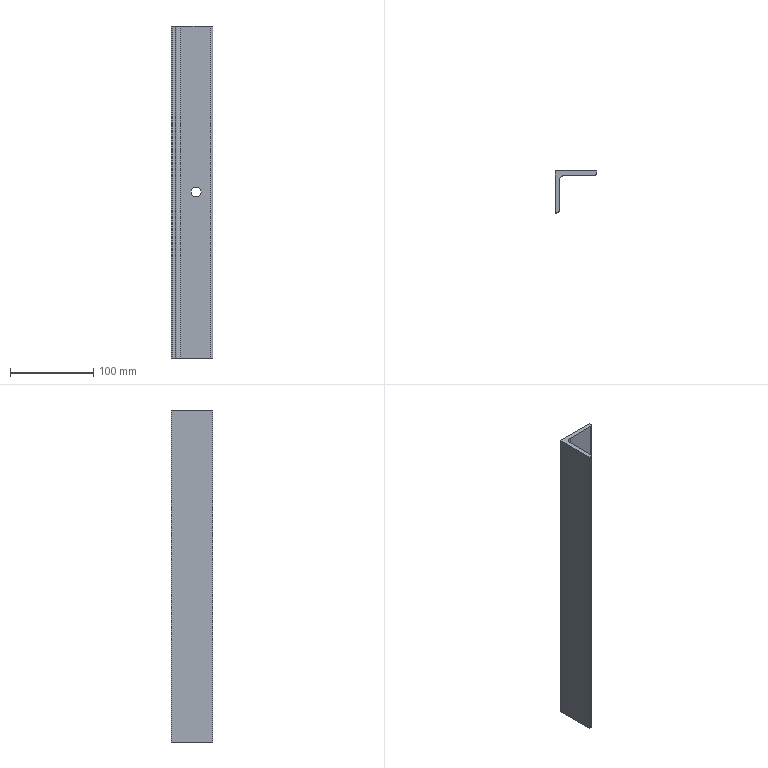Part | STEP file | Input 113 | 1 solid | 13 faces | box 50 x 50 x 400 mm | volume 191516 mm3 | plane 8 | cylinder 5 | commonest cylinder face diameters 6 x2 12 x2 13 x1
STEP:
#1=CARTESIAN_POINT('',(0.,0.,0.));
#2=DIRECTION('',(0.,0.,1.));
#3=DIRECTION('',(1.,0.,0.));
#4=AXIS2_PLACEMENT_3D('',#1,#2,#3);
#5=CARTESIAN_POINT('',(2984.,319.5,0.));
#6=VERTEX_POINT('',#5);
#7=CARTESIAN_POINT('',(2984.,324.5,0.));
#8=VERTEX_POINT('',#7);
#9=CARTESIAN_POINT('',(2984.,239.499,0.));
#10=DIRECTION('',(0.,1.,0.));
#11=VECTOR('',#10,1.);
#12=LINE('',#9,#11);
#13=CARTESIAN_POINT('',(2990.,239.499,0.));
#14=DIRECTION('',(0.,1.,0.));
#15=DIRECTION('',(-1.,0.,0.));
#16=AXIS2_PLACEMENT_3D('',#13,#14,#15);
#17=CYLINDRICAL_SURFACE('',#16,6.);
#18=CARTESIAN_POINT('',(6.283,0.));
#19=DIRECTION('',(0.,1.));
#20=VECTOR('',#19,1.);
#21=LINE('',#18,#20);
#22=(GEOMETRIC_REPRESENTATION_CONTEXT(2)PARAMETRIC_REPRESENTATION_CONTEXT()REPRESENTATION_CONTEXT('',''));
#23=DEFINITIONAL_REPRESENTATION('',(#21),#22);
#24=PCURVE('',#17,#23);
#25=CARTESIAN_POINT('',(2990.,239.499,0.));
#26=DIRECTION('',(0.,1.,0.));
#27=DIRECTION('',(-1.,0.,0.));
#28=AXIS2_PLACEMENT_3D('',#25,#26,#27);
#29=CYLINDRICAL_SURFACE('',#28,6.);
#30=CARTESIAN_POINT('',(0.,0.));
#31=DIRECTION('',(0.,1.));
#32=VECTOR('',#31,1.);
#33=LINE('',#30,#32);
#34=(GEOMETRIC_REPRESENTATION_CONTEXT(2)PARAMETRIC_REPRESENTATION_CONTEXT()REPRESENTATION_CONTEXT('',''));
#35=DEFINITIONAL_REPRESENTATION('',(#33),#34);
#36=PCURVE('',#29,#35);
#37=SURFACE_CURVE('',#12,(#24,#36),.PCURVE_S1.);
#38=EDGE_CURVE('',#6,#8,#37,.T.);
#39=ORIENTED_EDGE('',*,*,#38,.T.);
#40=CARTESIAN_POINT('',(2996.,324.5,0.));
#41=VERTEX_POINT('',#40);
#42=CARTESIAN_POINT('',(2990.,324.5,0.));
#43=DIRECTION('',(0.,1.,0.));
#44=DIRECTION('',(-1.,0.,0.));
#45=AXIS2_PLACEMENT_3D('',#42,#43,#44);
#46=CIRCLE('',#45,6.);
#47=CARTESIAN_POINT('',(0.,85.001));
#48=DIRECTION('',(1.,0.));
#49=VECTOR('',#48,1.);
#50=LINE('',#47,#49);
#51=(GEOMETRIC_REPRESENTATION_CONTEXT(2)PARAMETRIC_REPRESENTATION_CONTEXT()REPRESENTATION_CONTEXT('',''));
#52=DEFINITIONAL_REPRESENTATION('',(#50),#51);
#53=PCURVE('',#17,#52);
#54=CARTESIAN_POINT('',(3010.,324.5,200.));
#55=DIRECTION('',(0.,1.,0.));
#56=DIRECTION('',(-1.,0.,0.));
#57=AXIS2_PLACEMENT_3D('',#54,#55,#56);
#58=PLANE('',#57);
#59=CARTESIAN_POINT('',(20.,-200.));
#60=DIRECTION('',(1.,0.));
#61=AXIS2_PLACEMENT_2D('',#59,#60);
#62=CIRCLE('',#61,6.);
#63=(GEOMETRIC_REPRESENTATION_CONTEXT(2)PARAMETRIC_REPRESENTATION_CONTEXT()REPRESENTATION_CONTEXT('',''));
#64=DEFINITIONAL_REPRESENTATION('',(#62),#63);
#65=PCURVE('',#58,#64);
#66=SURFACE_CURVE('',#46,(#53,#65),.PCURVE_S1.);
#67=EDGE_CURVE('',#41,#8,#66,.T.);
#68=ORIENTED_EDGE('',*,*,#67,.F.);
#69=CARTESIAN_POINT('',(2996.,319.5,0.));
#70=VERTEX_POINT('',#69);
#71=CARTESIAN_POINT('',(2996.,239.499,0.));
#72=DIRECTION('',(0.,1.,0.));
#73=VECTOR('',#72,1.);
#74=LINE('',#71,#73);
#75=CARTESIAN_POINT('',(3.142,0.));
#76=DIRECTION('',(0.,1.));
#77=VECTOR('',#76,1.);
#78=LINE('',#75,#77);
#79=(GEOMETRIC_REPRESENTATION_CONTEXT(2)PARAMETRIC_REPRESENTATION_CONTEXT()REPRESENTATION_CONTEXT('',''));
#80=DEFINITIONAL_REPRESENTATION('',(#78),#79);
#81=PCURVE('',#17,#80);
#82=CARTESIAN_POINT('',(3.142,0.));
#83=DIRECTION('',(0.,1.));
#84=VECTOR('',#83,1.);
#85=LINE('',#82,#84);
#86=(GEOMETRIC_REPRESENTATION_CONTEXT(2)PARAMETRIC_REPRESENTATION_CONTEXT()REPRESENTATION_CONTEXT('',''));
#87=DEFINITIONAL_REPRESENTATION('',(#85),#86);
#88=PCURVE('',#29,#87);
#89=SURFACE_CURVE('',#74,(#81,#88),.PCURVE_S1.);
#90=EDGE_CURVE('',#70,#41,#89,.T.);
#91=ORIENTED_EDGE('',*,*,#90,.F.);
#92=CARTESIAN_POINT('',(2990.,319.5,0.));
#93=DIRECTION('',(0.,1.,0.));
#94=DIRECTION('',(1.,0.,0.));
#95=AXIS2_PLACEMENT_3D('',#92,#93,#94);
#96=CIRCLE('',#95,6.);
#97=CARTESIAN_POINT('',(3.142,80.001));
#98=DIRECTION('',(1.,0.));
#99=VECTOR('',#98,1.);
#100=LINE('',#97,#99);
#101=(GEOMETRIC_REPRESENTATION_CONTEXT(2)PARAMETRIC_REPRESENTATION_CONTEXT()REPRESENTATION_CONTEXT('',''));
#102=DEFINITIONAL_REPRESENTATION('',(#100),#101);
#103=PCURVE('',#17,#102);
#104=CARTESIAN_POINT('',(2971.5,319.5,200.));
#105=DIRECTION('',(0.,-1.,0.));
#106=DIRECTION('',(1.,0.,0.));
#107=AXIS2_PLACEMENT_3D('',#104,#105,#106);
#108=PLANE('',#107);
#109=CARTESIAN_POINT('',(24.5,-200.));
#110=CARTESIAN_POINT('',(24.5,-210.392));
#111=CARTESIAN_POINT('',(15.5,-205.196));
#112=CARTESIAN_POINT('',(6.5,-200.));
#113=CARTESIAN_POINT('',(15.5,-194.804));
#114=CARTESIAN_POINT('',(24.5,-189.608));
#115=CARTESIAN_POINT('',(24.5,-200.));
#116=(BOUNDED_CURVE()B_SPLINE_CURVE(2,(#109,#110,#111,#112,#113,#114,#115),.UNSPECIFIED.,.T.,.F.)B_SPLINE_CURVE_WITH_KNOTS((1,2,2,2,2,1),(-2.094,0.,2.094,4.189,6.283,8.378),.UNSPECIFIED.)CURVE()GEOMETRIC_REPRESENTATION_ITEM()RATIONAL_B_SPLINE_CURVE((1.,0.5,1.,0.5,1.,0.5,1.))REPRESENTATION_ITEM(''));
#117=(GEOMETRIC_REPRESENTATION_CONTEXT(2)PARAMETRIC_REPRESENTATION_CONTEXT()REPRESENTATION_CONTEXT('',''));
#118=DEFINITIONAL_REPRESENTATION('',(#116),#117);
#119=PCURVE('',#108,#118);
#120=SURFACE_CURVE('',#96,(#103,#119),.PCURVE_S1.);
#121=EDGE_CURVE('',#70,#6,#120,.T.);
#122=ORIENTED_EDGE('',*,*,#121,.T.);
#123=EDGE_LOOP('',(#39,#68,#91,#122));
#124=FACE_BOUND('',#123,.F.);
#125=ADVANCED_FACE('',(#124),#17,.F.);
#126=CARTESIAN_POINT('',(2990.,324.5,0.));
#127=DIRECTION('',(0.,1.,0.));
#128=DIRECTION('',(-1.,0.,0.));
#129=AXIS2_PLACEMENT_3D('',#126,#127,#128);
#130=CIRCLE('',#129,6.);
#131=CARTESIAN_POINT('',(20.,-200.));
#132=DIRECTION('',(1.,0.));
#133=AXIS2_PLACEMENT_2D('',#131,#132);
#134=CIRCLE('',#133,6.);
#135=(GEOMETRIC_REPRESENTATION_CONTEXT(2)PARAMETRIC_REPRESENTATION_CONTEXT()REPRESENTATION_CONTEXT('',''));
#136=DEFINITIONAL_REPRESENTATION('',(#134),#135);
#137=PCURVE('',#58,#136);
#138=CARTESIAN_POINT('',(0.,85.001));
#139=DIRECTION('',(1.,0.));
#140=VECTOR('',#139,1.);
#141=LINE('',#138,#140);
#142=(GEOMETRIC_REPRESENTATION_CONTEXT(2)PARAMETRIC_REPRESENTATION_CONTEXT()REPRESENTATION_CONTEXT('',''));
#143=DEFINITIONAL_REPRESENTATION('',(#141),#142);
#144=PCURVE('',#29,#143);
#145=SURFACE_CURVE('',#130,(#137,#144),.PCURVE_S1.);
#146=EDGE_CURVE('',#8,#41,#145,.T.);
#147=ORIENTED_EDGE('',*,*,#146,.F.);
#148=ORIENTED_EDGE('',*,*,#67,.F.);
#149=EDGE_LOOP('',(#147,#148));
#150=FACE_BOUND('',#149,.T.);
#151=CARTESIAN_POINT('',(2960.,324.5,-200.));
#152=VERTEX_POINT('',#151);
#153=CARTESIAN_POINT('',(3010.,324.5,-200.));
#154=VERTEX_POINT('',#153);
#155=CARTESIAN_POINT('',(3010.,324.5,-200.));
#156=DIRECTION('',(1.,0.,0.));
#157=VECTOR('',#156,1.);
#158=LINE('',#155,#157);
#159=CARTESIAN_POINT('',(0.,-400.));
#160=DIRECTION('',(-1.,0.));
#161=VECTOR('',#160,1.);
#162=LINE('',#159,#161);
#163=(GEOMETRIC_REPRESENTATION_CONTEXT(2)PARAMETRIC_REPRESENTATION_CONTEXT()REPRESENTATION_CONTEXT('',''));
#164=DEFINITIONAL_REPRESENTATION('',(#162),#163);
#165=PCURVE('',#58,#164);
#166=CARTESIAN_POINT('',(2962.,277.5,-200.));
#167=DIRECTION('',(0.,0.,1.));
#168=DIRECTION('',(1.,0.,0.));
#169=AXIS2_PLACEMENT_3D('',#166,#167,#168);
#170=PLANE('',#169);
#171=CARTESIAN_POINT('',(48.,47.));
#172=DIRECTION('',(1.,0.));
#173=VECTOR('',#172,1.);
#174=LINE('',#171,#173);
#175=(GEOMETRIC_REPRESENTATION_CONTEXT(2)PARAMETRIC_REPRESENTATION_CONTEXT()REPRESENTATION_CONTEXT('',''));
#176=DEFINITIONAL_REPRESENTATION('',(#174),#175);
#177=PCURVE('',#170,#176);
#178=SURFACE_CURVE('',#158,(#165,#177),.PCURVE_S1.);
#179=EDGE_CURVE('',#152,#154,#178,.T.);
#180=ORIENTED_EDGE('',*,*,#179,.F.);
#181=CARTESIAN_POINT('',(2960.,324.5,200.));
#182=VERTEX_POINT('',#181);
#183=CARTESIAN_POINT('',(2960.,324.5,200.));
#184=DIRECTION('',(0.,0.,-1.));
#185=VECTOR('',#184,1.);
#186=LINE('',#183,#185);
#187=CARTESIAN_POINT('',(50.,0.));
#188=DIRECTION('',(0.,-1.));
#189=VECTOR('',#188,1.);
#190=LINE('',#187,#189);
#191=(GEOMETRIC_REPRESENTATION_CONTEXT(2)PARAMETRIC_REPRESENTATION_CONTEXT()REPRESENTATION_CONTEXT('',''));
#192=DEFINITIONAL_REPRESENTATION('',(#190),#191);
#193=PCURVE('',#58,#192);
#194=CARTESIAN_POINT('',(2960.,324.5,200.));
#195=DIRECTION('',(-1.,0.,0.));
#196=DIRECTION('',(0.,0.,1.));
#197=AXIS2_PLACEMENT_3D('',#194,#195,#196);
#198=PLANE('',#197);
#199=CARTESIAN_POINT('',(0.,0.));
#200=DIRECTION('',(-1.,0.));
#201=VECTOR('',#200,1.);
#202=LINE('',#199,#201);
#203=(GEOMETRIC_REPRESENTATION_CONTEXT(2)PARAMETRIC_REPRESENTATION_CONTEXT()REPRESENTATION_CONTEXT('',''));
#204=DEFINITIONAL_REPRESENTATION('',(#202),#203);
#205=PCURVE('',#198,#204);
#206=SURFACE_CURVE('',#186,(#193,#205),.PCURVE_S1.);
#207=EDGE_CURVE('',#182,#152,#206,.T.);
#208=ORIENTED_EDGE('',*,*,#207,.F.);
#209=CARTESIAN_POINT('',(3010.,324.5,200.));
#210=VERTEX_POINT('',#209);
#211=CARTESIAN_POINT('',(3010.,324.5,200.));
#212=DIRECTION('',(1.,0.,0.));
#213=VECTOR('',#212,1.);
#214=LINE('',#211,#213);
#215=CARTESIAN_POINT('',(0.,0.));
#216=DIRECTION('',(-1.,0.));
#217=VECTOR('',#216,1.);
#218=LINE('',#215,#217);
#219=(GEOMETRIC_REPRESENTATION_CONTEXT(2)PARAMETRIC_REPRESENTATION_CONTEXT()REPRESENTATION_CONTEXT('',''));
#220=DEFINITIONAL_REPRESENTATION('',(#218),#219);
#221=PCURVE('',#58,#220);
#222=CARTESIAN_POINT('',(2962.,277.5,200.));
#223=DIRECTION('',(0.,0.,1.));
#224=DIRECTION('',(1.,0.,0.));
#225=AXIS2_PLACEMENT_3D('',#222,#223,#224);
#226=PLANE('',#225);
#227=CARTESIAN_POINT('',(48.,47.));
#228=DIRECTION('',(1.,0.));
#229=VECTOR('',#228,1.);
#230=LINE('',#227,#229);
#231=(GEOMETRIC_REPRESENTATION_CONTEXT(2)PARAMETRIC_REPRESENTATION_CONTEXT()REPRESENTATION_CONTEXT('',''));
#232=DEFINITIONAL_REPRESENTATION('',(#230),#231);
#233=PCURVE('',#226,#232);
#234=SURFACE_CURVE('',#214,(#221,#233),.PCURVE_S1.);
#235=EDGE_CURVE('',#182,#210,#234,.T.);
#236=ORIENTED_EDGE('',*,*,#235,.T.);
#237=CARTESIAN_POINT('',(3010.,324.5,200.));
#238=DIRECTION('',(0.,0.,-1.));
#239=VECTOR('',#238,1.);
#240=LINE('',#237,#239);
#241=CARTESIAN_POINT('',(0.,0.));
#242=DIRECTION('',(0.,-1.));
#243=VECTOR('',#242,1.);
#244=LINE('',#241,#243);
#245=(GEOMETRIC_REPRESENTATION_CONTEXT(2)PARAMETRIC_REPRESENTATION_CONTEXT()REPRESENTATION_CONTEXT('',''));
#246=DEFINITIONAL_REPRESENTATION('',(#244),#245);
#247=PCURVE('',#58,#246);
#248=CARTESIAN_POINT('',(3010.,324.5,200.));
#249=DIRECTION('',(1.,0.,0.));
#250=DIRECTION('',(0.,0.,-1.));
#251=AXIS2_PLACEMENT_3D('',#248,#249,#250);
#252=PLANE('',#251);
#253=CARTESIAN_POINT('',(0.,0.));
#254=DIRECTION('',(1.,0.));
#255=VECTOR('',#254,1.);
#256=LINE('',#253,#255);
#257=(GEOMETRIC_REPRESENTATION_CONTEXT(2)PARAMETRIC_REPRESENTATION_CONTEXT()REPRESENTATION_CONTEXT('',''));
#258=DEFINITIONAL_REPRESENTATION('',(#256),#257);
#259=PCURVE('',#252,#258);
#260=SURFACE_CURVE('',#240,(#247,#259),.PCURVE_S1.);
#261=EDGE_CURVE('',#210,#154,#260,.T.);
#262=ORIENTED_EDGE('',*,*,#261,.T.);
#263=EDGE_LOOP('',(#180,#208,#236,#262));
#264=FACE_BOUND('',#263,.T.);
#265=ADVANCED_FACE('',(#150,#264),#58,.T.);
#266=CARTESIAN_POINT('',(2960.,274.5,-200.));
#267=VERTEX_POINT('',#266);
#268=CARTESIAN_POINT('',(2960.,324.5,-200.));
#269=DIRECTION('',(0.,1.,0.));
#270=VECTOR('',#269,1.);
#271=LINE('',#268,#270);
#272=CARTESIAN_POINT('',(-400.,0.));
#273=DIRECTION('',(0.,1.));
#274=VECTOR('',#273,1.);
#275=LINE('',#272,#274);
#276=(GEOMETRIC_REPRESENTATION_CONTEXT(2)PARAMETRIC_REPRESENTATION_CONTEXT()REPRESENTATION_CONTEXT('',''));
#277=DEFINITIONAL_REPRESENTATION('',(#275),#276);
#278=PCURVE('',#198,#277);
#279=CARTESIAN_POINT('',(-2.,47.));
#280=DIRECTION('',(0.,1.));
#281=VECTOR('',#280,1.);
#282=LINE('',#279,#281);
#283=(GEOMETRIC_REPRESENTATION_CONTEXT(2)PARAMETRIC_REPRESENTATION_CONTEXT()REPRESENTATION_CONTEXT('',''));
#284=DEFINITIONAL_REPRESENTATION('',(#282),#283);
#285=PCURVE('',#170,#284);
#286=SURFACE_CURVE('',#271,(#278,#285),.PCURVE_S1.);
#287=EDGE_CURVE('',#267,#152,#286,.T.);
#288=ORIENTED_EDGE('',*,*,#287,.F.);
#289=CARTESIAN_POINT('',(2960.,274.5,200.));
#290=VERTEX_POINT('',#289);
#291=CARTESIAN_POINT('',(2960.,274.5,200.));
#292=DIRECTION('',(0.,0.,-1.));
#293=VECTOR('',#292,1.);
#294=LINE('',#291,#293);
#295=CARTESIAN_POINT('',(0.,-50.));
#296=DIRECTION('',(-1.,0.));
#297=VECTOR('',#296,1.);
#298=LINE('',#295,#297);
#299=(GEOMETRIC_REPRESENTATION_CONTEXT(2)PARAMETRIC_REPRESENTATION_CONTEXT()REPRESENTATION_CONTEXT('',''));
#300=DEFINITIONAL_REPRESENTATION('',(#298),#299);
#301=PCURVE('',#198,#300);
#302=CARTESIAN_POINT('',(2960.,274.5,200.));
#303=DIRECTION('',(0.,-1.,0.));
#304=DIRECTION('',(1.,0.,0.));
#305=AXIS2_PLACEMENT_3D('',#302,#303,#304);
#306=PLANE('',#305);
#307=CARTESIAN_POINT('',(0.,0.));
#308=DIRECTION('',(0.,-1.));
#309=VECTOR('',#308,1.);
#310=LINE('',#307,#309);
#311=(GEOMETRIC_REPRESENTATION_CONTEXT(2)PARAMETRIC_REPRESENTATION_CONTEXT()REPRESENTATION_CONTEXT('',''));
#312=DEFINITIONAL_REPRESENTATION('',(#310),#311);
#313=PCURVE('',#306,#312);
#314=SURFACE_CURVE('',#294,(#301,#313),.PCURVE_S1.);
#315=EDGE_CURVE('',#290,#267,#314,.T.);
#316=ORIENTED_EDGE('',*,*,#315,.F.);
#317=CARTESIAN_POINT('',(2960.,324.5,200.));
#318=DIRECTION('',(0.,1.,0.));
#319=VECTOR('',#318,1.);
#320=LINE('',#317,#319);
#321=CARTESIAN_POINT('',(0.,0.));
#322=DIRECTION('',(0.,1.));
#323=VECTOR('',#322,1.);
#324=LINE('',#321,#323);
#325=(GEOMETRIC_REPRESENTATION_CONTEXT(2)PARAMETRIC_REPRESENTATION_CONTEXT()REPRESENTATION_CONTEXT('',''));
#326=DEFINITIONAL_REPRESENTATION('',(#324),#325);
#327=PCURVE('',#198,#326);
#328=CARTESIAN_POINT('',(-2.,47.));
#329=DIRECTION('',(0.,1.));
#330=VECTOR('',#329,1.);
#331=LINE('',#328,#330);
#332=(GEOMETRIC_REPRESENTATION_CONTEXT(2)PARAMETRIC_REPRESENTATION_CONTEXT()REPRESENTATION_CONTEXT('',''));
#333=DEFINITIONAL_REPRESENTATION('',(#331),#332);
#334=PCURVE('',#226,#333);
#335=SURFACE_CURVE('',#320,(#327,#334),.PCURVE_S1.);
#336=EDGE_CURVE('',#290,#182,#335,.T.);
#337=ORIENTED_EDGE('',*,*,#336,.T.);
#338=ORIENTED_EDGE('',*,*,#207,.T.);
#339=EDGE_LOOP('',(#288,#316,#337,#338));
#340=FACE_BOUND('',#339,.T.);
#341=ADVANCED_FACE('',(#340),#198,.T.);
#342=CARTESIAN_POINT('',(2962.,274.5,-200.));
#343=VERTEX_POINT('',#342);
#344=CARTESIAN_POINT('',(2960.,274.5,-200.));
#345=DIRECTION('',(-1.,0.,0.));
#346=VECTOR('',#345,1.);
#347=LINE('',#344,#346);
#348=CARTESIAN_POINT('',(0.,-400.));
#349=DIRECTION('',(-1.,0.));
#350=VECTOR('',#349,1.);
#351=LINE('',#348,#350);
#352=(GEOMETRIC_REPRESENTATION_CONTEXT(2)PARAMETRIC_REPRESENTATION_CONTEXT()REPRESENTATION_CONTEXT('',''));
#353=DEFINITIONAL_REPRESENTATION('',(#351),#352);
#354=PCURVE('',#306,#353);
#355=CARTESIAN_POINT('',(-2.,-3.));
#356=DIRECTION('',(-1.,0.));
#357=VECTOR('',#356,1.);
#358=LINE('',#355,#357);
#359=(GEOMETRIC_REPRESENTATION_CONTEXT(2)PARAMETRIC_REPRESENTATION_CONTEXT()REPRESENTATION_CONTEXT('',''));
#360=DEFINITIONAL_REPRESENTATION('',(#358),#359);
#361=PCURVE('',#170,#360);
#362=SURFACE_CURVE('',#347,(#354,#361),.PCURVE_S1.);
#363=EDGE_CURVE('',#343,#267,#362,.T.);
#364=ORIENTED_EDGE('',*,*,#363,.F.);
#365=CARTESIAN_POINT('',(2962.,274.5,200.));
#366=VERTEX_POINT('',#365);
#367=CARTESIAN_POINT('',(2962.,274.5,200.));
#368=DIRECTION('',(0.,0.,-1.));
#369=VECTOR('',#368,1.);
#370=LINE('',#367,#369);
#371=CARTESIAN_POINT('',(2.,0.));
#372=DIRECTION('',(0.,-1.));
#373=VECTOR('',#372,1.);
#374=LINE('',#371,#373);
#375=(GEOMETRIC_REPRESENTATION_CONTEXT(2)PARAMETRIC_REPRESENTATION_CONTEXT()REPRESENTATION_CONTEXT('',''));
#376=DEFINITIONAL_REPRESENTATION('',(#374),#375);
#377=PCURVE('',#306,#376);
#378=CARTESIAN_POINT('',(2962.,277.5,200.));
#379=DIRECTION('',(0.,0.,-1.));
#380=DIRECTION('',(-1.,0.,0.));
#381=AXIS2_PLACEMENT_3D('',#378,#379,#380);
#382=CYLINDRICAL_SURFACE('',#381,3.);
#383=CARTESIAN_POINT('',(4.712,0.));
#384=DIRECTION('',(0.,1.));
#385=VECTOR('',#384,1.);
#386=LINE('',#383,#385);
#387=(GEOMETRIC_REPRESENTATION_CONTEXT(2)PARAMETRIC_REPRESENTATION_CONTEXT()REPRESENTATION_CONTEXT('',''));
#388=DEFINITIONAL_REPRESENTATION('',(#386),#387);
#389=PCURVE('',#382,#388);
#390=SURFACE_CURVE('',#370,(#377,#389),.PCURVE_S1.);
#391=EDGE_CURVE('',#366,#343,#390,.T.);
#392=ORIENTED_EDGE('',*,*,#391,.F.);
#393=CARTESIAN_POINT('',(2960.,274.5,200.));
#394=DIRECTION('',(-1.,0.,0.));
#395=VECTOR('',#394,1.);
#396=LINE('',#393,#395);
#397=CARTESIAN_POINT('',(0.,0.));
#398=DIRECTION('',(-1.,0.));
#399=VECTOR('',#398,1.);
#400=LINE('',#397,#399);
#401=(GEOMETRIC_REPRESENTATION_CONTEXT(2)PARAMETRIC_REPRESENTATION_CONTEXT()REPRESENTATION_CONTEXT('',''));
#402=DEFINITIONAL_REPRESENTATION('',(#400),#401);
#403=PCURVE('',#306,#402);
#404=CARTESIAN_POINT('',(-2.,-3.));
#405=DIRECTION('',(-1.,0.));
#406=VECTOR('',#405,1.);
#407=LINE('',#404,#406);
#408=(GEOMETRIC_REPRESENTATION_CONTEXT(2)PARAMETRIC_REPRESENTATION_CONTEXT()REPRESENTATION_CONTEXT('',''));
#409=DEFINITIONAL_REPRESENTATION('',(#407),#408);
#410=PCURVE('',#226,#409);
#411=SURFACE_CURVE('',#396,(#403,#410),.PCURVE_S1.);
#412=EDGE_CURVE('',#366,#290,#411,.T.);
#413=ORIENTED_EDGE('',*,*,#412,.T.);
#414=ORIENTED_EDGE('',*,*,#315,.T.);
#415=EDGE_LOOP('',(#364,#392,#413,#414));
#416=FACE_BOUND('',#415,.T.);
#417=ADVANCED_FACE('',(#416),#306,.T.);
#418=CARTESIAN_POINT('',(2965.,277.5,-200.));
#419=VERTEX_POINT('',#418);
#420=CARTESIAN_POINT('',(2962.,277.5,-200.));
#421=DIRECTION('',(0.,0.,-1.));
#422=DIRECTION('',(1.,0.,0.));
#423=AXIS2_PLACEMENT_3D('',#420,#421,#422);
#424=CIRCLE('',#423,3.);
#425=CARTESIAN_POINT('',(3.142,400.));
#426=DIRECTION('',(1.,0.));
#427=VECTOR('',#426,1.);
#428=LINE('',#425,#427);
#429=(GEOMETRIC_REPRESENTATION_CONTEXT(2)PARAMETRIC_REPRESENTATION_CONTEXT()REPRESENTATION_CONTEXT('',''));
#430=DEFINITIONAL_REPRESENTATION('',(#428),#429);
#431=PCURVE('',#382,#430);
#432=CARTESIAN_POINT('',(3.,0.));
#433=CARTESIAN_POINT('',(3.,-5.196));
#434=CARTESIAN_POINT('',(-1.5,-2.598));
#435=CARTESIAN_POINT('',(-6.,0.));
#436=CARTESIAN_POINT('',(-1.5,2.598));
#437=CARTESIAN_POINT('',(3.,5.196));
#438=CARTESIAN_POINT('',(3.,0.));
#439=(BOUNDED_CURVE()B_SPLINE_CURVE(2,(#432,#433,#434,#435,#436,#437,#438),.UNSPECIFIED.,.T.,.F.)B_SPLINE_CURVE_WITH_KNOTS((1,2,2,2,2,1),(-2.094,0.,2.094,4.189,6.283,8.378),.UNSPECIFIED.)CURVE()GEOMETRIC_REPRESENTATION_ITEM()RATIONAL_B_SPLINE_CURVE((1.,0.5,1.,0.5,1.,0.5,1.))REPRESENTATION_ITEM(''));
#440=(GEOMETRIC_REPRESENTATION_CONTEXT(2)PARAMETRIC_REPRESENTATION_CONTEXT()REPRESENTATION_CONTEXT('',''));
#441=DEFINITIONAL_REPRESENTATION('',(#439),#440);
#442=PCURVE('',#170,#441);
#443=SURFACE_CURVE('',#424,(#431,#442),.PCURVE_S1.);
#444=EDGE_CURVE('',#419,#343,#443,.T.);
#445=ORIENTED_EDGE('',*,*,#444,.F.);
#446=CARTESIAN_POINT('',(2965.,277.5,200.));
#447=VERTEX_POINT('',#446);
#448=CARTESIAN_POINT('',(2965.,277.5,200.));
#449=DIRECTION('',(0.,0.,-1.));
#450=VECTOR('',#449,1.);
#451=LINE('',#448,#450);
#452=CARTESIAN_POINT('',(3.142,0.));
#453=DIRECTION('',(0.,1.));
#454=VECTOR('',#453,1.);
#455=LINE('',#452,#454);
#456=(GEOMETRIC_REPRESENTATION_CONTEXT(2)PARAMETRIC_REPRESENTATION_CONTEXT()REPRESENTATION_CONTEXT('',''));
#457=DEFINITIONAL_REPRESENTATION('',(#455),#456);
#458=PCURVE('',#382,#457);
#459=CARTESIAN_POINT('',(2965.,277.5,200.));
#460=DIRECTION('',(1.,0.,0.));
#461=DIRECTION('',(0.,0.,-1.));
#462=AXIS2_PLACEMENT_3D('',#459,#460,#461);
#463=PLANE('',#462);
#464=CARTESIAN_POINT('',(0.,0.));
#465=DIRECTION('',(1.,0.));
#466=VECTOR('',#465,1.);
#467=LINE('',#464,#466);
#468=(GEOMETRIC_REPRESENTATION_CONTEXT(2)PARAMETRIC_REPRESENTATION_CONTEXT()REPRESENTATION_CONTEXT('',''));
#469=DEFINITIONAL_REPRESENTATION('',(#467),#468);
#470=PCURVE('',#463,#469);
#471=SURFACE_CURVE('',#451,(#458,#470),.PCURVE_S1.);
#472=EDGE_CURVE('',#447,#419,#471,.T.);
#473=ORIENTED_EDGE('',*,*,#472,.F.);
#474=CARTESIAN_POINT('',(2962.,277.5,200.));
#475=DIRECTION('',(0.,0.,-1.));
#476=DIRECTION('',(1.,0.,0.));
#477=AXIS2_PLACEMENT_3D('',#474,#475,#476);
#478=CIRCLE('',#477,3.);
#479=CARTESIAN_POINT('',(3.142,0.));
#480=DIRECTION('',(1.,0.));
#481=VECTOR('',#480,1.);
#482=LINE('',#479,#481);
#483=(GEOMETRIC_REPRESENTATION_CONTEXT(2)PARAMETRIC_REPRESENTATION_CONTEXT()REPRESENTATION_CONTEXT('',''));
#484=DEFINITIONAL_REPRESENTATION('',(#482),#483);
#485=PCURVE('',#382,#484);
#486=CARTESIAN_POINT('',(3.,0.));
#487=CARTESIAN_POINT('',(3.,-5.196));
#488=CARTESIAN_POINT('',(-1.5,-2.598));
#489=CARTESIAN_POINT('',(-6.,0.));
#490=CARTESIAN_POINT('',(-1.5,2.598));
#491=CARTESIAN_POINT('',(3.,5.196));
#492=CARTESIAN_POINT('',(3.,0.));
#493=(BOUNDED_CURVE()B_SPLINE_CURVE(2,(#486,#487,#488,#489,#490,#491,#492),.UNSPECIFIED.,.T.,.F.)B_SPLINE_CURVE_WITH_KNOTS((1,2,2,2,2,1),(-2.094,0.,2.094,4.189,6.283,8.378),.UNSPECIFIED.)CURVE()GEOMETRIC_REPRESENTATION_ITEM()RATIONAL_B_SPLINE_CURVE((1.,0.5,1.,0.5,1.,0.5,1.))REPRESENTATION_ITEM(''));
#494=(GEOMETRIC_REPRESENTATION_CONTEXT(2)PARAMETRIC_REPRESENTATION_CONTEXT()REPRESENTATION_CONTEXT('',''));
#495=DEFINITIONAL_REPRESENTATION('',(#493),#494);
#496=PCURVE('',#226,#495);
#497=SURFACE_CURVE('',#478,(#485,#496),.PCURVE_S1.);
#498=EDGE_CURVE('',#447,#366,#497,.T.);
#499=ORIENTED_EDGE('',*,*,#498,.T.);
#500=ORIENTED_EDGE('',*,*,#391,.T.);
#501=EDGE_LOOP('',(#445,#473,#499,#500));
#502=FACE_BOUND('',#501,.T.);
#503=ADVANCED_FACE('',(#502),#382,.T.);
#504=CARTESIAN_POINT('',(2965.,313.,-200.));
#505=VERTEX_POINT('',#504);
#506=CARTESIAN_POINT('',(2965.,277.5,-200.));
#507=DIRECTION('',(0.,-1.,0.));
#508=VECTOR('',#507,1.);
#509=LINE('',#506,#508);
#510=CARTESIAN_POINT('',(400.,0.));
#511=DIRECTION('',(0.,-1.));
#512=VECTOR('',#511,1.);
#513=LINE('',#510,#512);
#514=(GEOMETRIC_REPRESENTATION_CONTEXT(2)PARAMETRIC_REPRESENTATION_CONTEXT()REPRESENTATION_CONTEXT('',''));
#515=DEFINITIONAL_REPRESENTATION('',(#513),#514);
#516=PCURVE('',#463,#515);
#517=CARTESIAN_POINT('',(3.,0.));
#518=DIRECTION('',(0.,-1.));
#519=VECTOR('',#518,1.);
#520=LINE('',#517,#519);
#521=(GEOMETRIC_REPRESENTATION_CONTEXT(2)PARAMETRIC_REPRESENTATION_CONTEXT()REPRESENTATION_CONTEXT('',''));
#522=DEFINITIONAL_REPRESENTATION('',(#520),#521);
#523=PCURVE('',#170,#522);
#524=SURFACE_CURVE('',#509,(#516,#523),.PCURVE_S1.);
#525=EDGE_CURVE('',#505,#419,#524,.T.);
#526=ORIENTED_EDGE('',*,*,#525,.F.);
#527=CARTESIAN_POINT('',(2965.,313.,200.));
#528=VERTEX_POINT('',#527);
#529=CARTESIAN_POINT('',(2965.,313.,200.));
#530=DIRECTION('',(0.,0.,-1.));
#531=VECTOR('',#530,1.);
#532=LINE('',#529,#531);
#533=CARTESIAN_POINT('',(0.,35.5));
#534=DIRECTION('',(1.,0.));
#535=VECTOR('',#534,1.);
#536=LINE('',#533,#535);
#537=(GEOMETRIC_REPRESENTATION_CONTEXT(2)PARAMETRIC_REPRESENTATION_CONTEXT()REPRESENTATION_CONTEXT('',''));
#538=DEFINITIONAL_REPRESENTATION('',(#536),#537);
#539=PCURVE('',#463,#538);
#540=CARTESIAN_POINT('',(2971.5,313.,200.));
#541=DIRECTION('',(0.,0.,-1.));
#542=DIRECTION('',(-1.,0.,0.));
#543=AXIS2_PLACEMENT_3D('',#540,#541,#542);
#544=CYLINDRICAL_SURFACE('',#543,6.5);
#545=CARTESIAN_POINT('',(0.,0.));
#546=DIRECTION('',(0.,1.));
#547=VECTOR('',#546,1.);
#548=LINE('',#545,#547);
#549=(GEOMETRIC_REPRESENTATION_CONTEXT(2)PARAMETRIC_REPRESENTATION_CONTEXT()REPRESENTATION_CONTEXT('',''));
#550=DEFINITIONAL_REPRESENTATION('',(#548),#549);
#551=PCURVE('',#544,#550);
#552=SURFACE_CURVE('',#532,(#539,#551),.PCURVE_S1.);
#553=EDGE_CURVE('',#528,#505,#552,.T.);
#554=ORIENTED_EDGE('',*,*,#553,.F.);
#555=CARTESIAN_POINT('',(2965.,277.5,200.));
#556=DIRECTION('',(0.,-1.,0.));
#557=VECTOR('',#556,1.);
#558=LINE('',#555,#557);
#559=CARTESIAN_POINT('',(0.,0.));
#560=DIRECTION('',(0.,-1.));
#561=VECTOR('',#560,1.);
#562=LINE('',#559,#561);
#563=(GEOMETRIC_REPRESENTATION_CONTEXT(2)PARAMETRIC_REPRESENTATION_CONTEXT()REPRESENTATION_CONTEXT('',''));
#564=DEFINITIONAL_REPRESENTATION('',(#562),#563);
#565=PCURVE('',#463,#564);
#566=CARTESIAN_POINT('',(3.,0.));
#567=DIRECTION('',(0.,-1.));
#568=VECTOR('',#567,1.);
#569=LINE('',#566,#568);
#570=(GEOMETRIC_REPRESENTATION_CONTEXT(2)PARAMETRIC_REPRESENTATION_CONTEXT()REPRESENTATION_CONTEXT('',''));
#571=DEFINITIONAL_REPRESENTATION('',(#569),#570);
#572=PCURVE('',#226,#571);
#573=SURFACE_CURVE('',#558,(#565,#572),.PCURVE_S1.);
#574=EDGE_CURVE('',#528,#447,#573,.T.);
#575=ORIENTED_EDGE('',*,*,#574,.T.);
#576=ORIENTED_EDGE('',*,*,#472,.T.);
#577=EDGE_LOOP('',(#526,#554,#575,#576));
#578=FACE_BOUND('',#577,.T.);
#579=ADVANCED_FACE('',(#578),#463,.T.);
#580=ORIENTED_EDGE('',*,*,#553,.F.);
#581=CARTESIAN_POINT('',(2971.5,319.5,200.));
#582=VERTEX_POINT('',#581);
#583=CARTESIAN_POINT('',(2971.5,313.,200.));
#584=DIRECTION('',(0.,0.,1.));
#585=DIRECTION('',(1.,0.,0.));
#586=AXIS2_PLACEMENT_3D('',#583,#584,#585);
#587=CIRCLE('',#586,6.5);
#588=CARTESIAN_POINT('',(3.142,0.));
#589=DIRECTION('',(-1.,0.));
#590=VECTOR('',#589,1.);
#591=LINE('',#588,#590);
#592=(GEOMETRIC_REPRESENTATION_CONTEXT(2)PARAMETRIC_REPRESENTATION_CONTEXT()REPRESENTATION_CONTEXT('',''));
#593=DEFINITIONAL_REPRESENTATION('',(#591),#592);
#594=PCURVE('',#544,#593);
#595=CARTESIAN_POINT('',(9.5,35.5));
#596=DIRECTION('',(1.,0.));
#597=AXIS2_PLACEMENT_2D('',#595,#596);
#598=CIRCLE('',#597,6.5);
#599=(GEOMETRIC_REPRESENTATION_CONTEXT(2)PARAMETRIC_REPRESENTATION_CONTEXT()REPRESENTATION_CONTEXT('',''));
#600=DEFINITIONAL_REPRESENTATION('',(#598),#599);
#601=PCURVE('',#226,#600);
#602=SURFACE_CURVE('',#587,(#594,#601),.PCURVE_S1.);
#603=EDGE_CURVE('',#582,#528,#602,.T.);
#604=ORIENTED_EDGE('',*,*,#603,.F.);
#605=CARTESIAN_POINT('',(2971.5,319.5,-200.));
#606=VERTEX_POINT('',#605);
#607=CARTESIAN_POINT('',(2971.5,319.5,200.));
#608=DIRECTION('',(0.,0.,-1.));
#609=VECTOR('',#608,1.);
#610=LINE('',#607,#609);
#611=CARTESIAN_POINT('',(1.571,0.));
#612=DIRECTION('',(0.,1.));
#613=VECTOR('',#612,1.);
#614=LINE('',#611,#613);
#615=(GEOMETRIC_REPRESENTATION_CONTEXT(2)PARAMETRIC_REPRESENTATION_CONTEXT()REPRESENTATION_CONTEXT('',''));
#616=DEFINITIONAL_REPRESENTATION('',(#614),#615);
#617=PCURVE('',#544,#616);
#618=CARTESIAN_POINT('',(0.,0.));
#619=DIRECTION('',(0.,-1.));
#620=VECTOR('',#619,1.);
#621=LINE('',#618,#620);
#622=(GEOMETRIC_REPRESENTATION_CONTEXT(2)PARAMETRIC_REPRESENTATION_CONTEXT()REPRESENTATION_CONTEXT('',''));
#623=DEFINITIONAL_REPRESENTATION('',(#621),#622);
#624=PCURVE('',#108,#623);
#625=SURFACE_CURVE('',#610,(#617,#624),.PCURVE_S1.);
#626=EDGE_CURVE('',#582,#606,#625,.T.);
#627=ORIENTED_EDGE('',*,*,#626,.T.);
#628=CARTESIAN_POINT('',(2971.5,313.,-200.));
#629=DIRECTION('',(0.,0.,1.));
#630=DIRECTION('',(1.,0.,0.));
#631=AXIS2_PLACEMENT_3D('',#628,#629,#630);
#632=CIRCLE('',#631,6.5);
#633=CARTESIAN_POINT('',(3.142,400.));
#634=DIRECTION('',(-1.,0.));
#635=VECTOR('',#634,1.);
#636=LINE('',#633,#635);
#637=(GEOMETRIC_REPRESENTATION_CONTEXT(2)PARAMETRIC_REPRESENTATION_CONTEXT()REPRESENTATION_CONTEXT('',''));
#638=DEFINITIONAL_REPRESENTATION('',(#636),#637);
#639=PCURVE('',#544,#638);
#640=CARTESIAN_POINT('',(9.5,35.5));
#641=DIRECTION('',(1.,0.));
#642=AXIS2_PLACEMENT_2D('',#640,#641);
#643=CIRCLE('',#642,6.5);
#644=(GEOMETRIC_REPRESENTATION_CONTEXT(2)PARAMETRIC_REPRESENTATION_CONTEXT()REPRESENTATION_CONTEXT('',''));
#645=DEFINITIONAL_REPRESENTATION('',(#643),#644);
#646=PCURVE('',#170,#645);
#647=SURFACE_CURVE('',#632,(#639,#646),.PCURVE_S1.);
#648=EDGE_CURVE('',#606,#505,#647,.T.);
#649=ORIENTED_EDGE('',*,*,#648,.T.);
#650=EDGE_LOOP('',(#580,#604,#627,#649));
#651=FACE_BOUND('',#650,.F.);
#652=ADVANCED_FACE('',(#651),#544,.F.);
#653=CARTESIAN_POINT('',(2990.,319.5,0.));
#654=DIRECTION('',(0.,1.,0.));
#655=DIRECTION('',(1.,0.,0.));
#656=AXIS2_PLACEMENT_3D('',#653,#654,#655);
#657=CIRCLE('',#656,6.);
#658=CARTESIAN_POINT('',(24.5,-200.));
#659=CARTESIAN_POINT('',(24.5,-210.392));
#660=CARTESIAN_POINT('',(15.5,-205.196));
#661=CARTESIAN_POINT('',(6.5,-200.));
#662=CARTESIAN_POINT('',(15.5,-194.804));
#663=CARTESIAN_POINT('',(24.5,-189.608));
#664=CARTESIAN_POINT('',(24.5,-200.));
#665=(BOUNDED_CURVE()B_SPLINE_CURVE(2,(#658,#659,#660,#661,#662,#663,#664),.UNSPECIFIED.,.T.,.F.)B_SPLINE_CURVE_WITH_KNOTS((1,2,2,2,2,1),(-2.094,0.,2.094,4.189,6.283,8.378),.UNSPECIFIED.)CURVE()GEOMETRIC_REPRESENTATION_ITEM()RATIONAL_B_SPLINE_CURVE((1.,0.5,1.,0.5,1.,0.5,1.))REPRESENTATION_ITEM(''));
#666=(GEOMETRIC_REPRESENTATION_CONTEXT(2)PARAMETRIC_REPRESENTATION_CONTEXT()REPRESENTATION_CONTEXT('',''));
#667=DEFINITIONAL_REPRESENTATION('',(#665),#666);
#668=PCURVE('',#108,#667);
#669=CARTESIAN_POINT('',(-3.142,80.001));
#670=DIRECTION('',(1.,0.));
#671=VECTOR('',#670,1.);
#672=LINE('',#669,#671);
#673=(GEOMETRIC_REPRESENTATION_CONTEXT(2)PARAMETRIC_REPRESENTATION_CONTEXT()REPRESENTATION_CONTEXT('',''));
#674=DEFINITIONAL_REPRESENTATION('',(#672),#673);
#675=PCURVE('',#29,#674);
#676=SURFACE_CURVE('',#657,(#668,#675),.PCURVE_S1.);
#677=EDGE_CURVE('',#6,#70,#676,.T.);
#678=ORIENTED_EDGE('',*,*,#677,.T.);
#679=ORIENTED_EDGE('',*,*,#121,.T.);
#680=EDGE_LOOP('',(#678,#679));
#681=FACE_BOUND('',#680,.T.);
#682=CARTESIAN_POINT('',(3007.,319.5,-200.));
#683=VERTEX_POINT('',#682);
#684=CARTESIAN_POINT('',(2971.5,319.5,-200.));
#685=DIRECTION('',(-1.,0.,0.));
#686=VECTOR('',#685,1.);
#687=LINE('',#684,#686);
#688=CARTESIAN_POINT('',(0.,-400.));
#689=DIRECTION('',(-1.,0.));
#690=VECTOR('',#689,1.);
#691=LINE('',#688,#690);
#692=(GEOMETRIC_REPRESENTATION_CONTEXT(2)PARAMETRIC_REPRESENTATION_CONTEXT()REPRESENTATION_CONTEXT('',''));
#693=DEFINITIONAL_REPRESENTATION('',(#691),#692);
#694=PCURVE('',#108,#693);
#695=CARTESIAN_POINT('',(9.5,42.));
#696=DIRECTION('',(-1.,0.));
#697=VECTOR('',#696,1.);
#698=LINE('',#695,#697);
#699=(GEOMETRIC_REPRESENTATION_CONTEXT(2)PARAMETRIC_REPRESENTATION_CONTEXT()REPRESENTATION_CONTEXT('',''));
#700=DEFINITIONAL_REPRESENTATION('',(#698),#699);
#701=PCURVE('',#170,#700);
#702=SURFACE_CURVE('',#687,(#694,#701),.PCURVE_S1.);
#703=EDGE_CURVE('',#683,#606,#702,.T.);
#704=ORIENTED_EDGE('',*,*,#703,.F.);
#705=CARTESIAN_POINT('',(3007.,319.5,200.));
#706=VERTEX_POINT('',#705);
#707=CARTESIAN_POINT('',(3007.,319.5,200.));
#708=DIRECTION('',(0.,0.,-1.));
#709=VECTOR('',#708,1.);
#710=LINE('',#707,#709);
#711=CARTESIAN_POINT('',(35.5,0.));
#712=DIRECTION('',(0.,-1.));
#713=VECTOR('',#712,1.);
#714=LINE('',#711,#713);
#715=(GEOMETRIC_REPRESENTATION_CONTEXT(2)PARAMETRIC_REPRESENTATION_CONTEXT()REPRESENTATION_CONTEXT('',''));
#716=DEFINITIONAL_REPRESENTATION('',(#714),#715);
#717=PCURVE('',#108,#716);
#718=CARTESIAN_POINT('',(3007.,322.5,200.));
#719=DIRECTION('',(0.,0.,-1.));
#720=DIRECTION('',(-1.,0.,0.));
#721=AXIS2_PLACEMENT_3D('',#718,#719,#720);
#722=CYLINDRICAL_SURFACE('',#721,3.);
#723=CARTESIAN_POINT('',(4.712,0.));
#724=DIRECTION('',(0.,1.));
#725=VECTOR('',#724,1.);
#726=LINE('',#723,#725);
#727=(GEOMETRIC_REPRESENTATION_CONTEXT(2)PARAMETRIC_REPRESENTATION_CONTEXT()REPRESENTATION_CONTEXT('',''));
#728=DEFINITIONAL_REPRESENTATION('',(#726),#727);
#729=PCURVE('',#722,#728);
#730=SURFACE_CURVE('',#710,(#717,#729),.PCURVE_S1.);
#731=EDGE_CURVE('',#706,#683,#730,.T.);
#732=ORIENTED_EDGE('',*,*,#731,.F.);
#733=CARTESIAN_POINT('',(2971.5,319.5,200.));
#734=DIRECTION('',(-1.,0.,0.));
#735=VECTOR('',#734,1.);
#736=LINE('',#733,#735);
#737=CARTESIAN_POINT('',(0.,0.));
#738=DIRECTION('',(-1.,0.));
#739=VECTOR('',#738,1.);
#740=LINE('',#737,#739);
#741=(GEOMETRIC_REPRESENTATION_CONTEXT(2)PARAMETRIC_REPRESENTATION_CONTEXT()REPRESENTATION_CONTEXT('',''));
#742=DEFINITIONAL_REPRESENTATION('',(#740),#741);
#743=PCURVE('',#108,#742);
#744=CARTESIAN_POINT('',(9.5,42.));
#745=DIRECTION('',(-1.,0.));
#746=VECTOR('',#745,1.);
#747=LINE('',#744,#746);
#748=(GEOMETRIC_REPRESENTATION_CONTEXT(2)PARAMETRIC_REPRESENTATION_CONTEXT()REPRESENTATION_CONTEXT('',''));
#749=DEFINITIONAL_REPRESENTATION('',(#747),#748);
#750=PCURVE('',#226,#749);
#751=SURFACE_CURVE('',#736,(#743,#750),.PCURVE_S1.);
#752=EDGE_CURVE('',#706,#582,#751,.T.);
#753=ORIENTED_EDGE('',*,*,#752,.T.);
#754=ORIENTED_EDGE('',*,*,#626,.T.);
#755=EDGE_LOOP('',(#704,#732,#753,#754));
#756=FACE_BOUND('',#755,.T.);
#757=ADVANCED_FACE('',(#681,#756),#108,.T.);
#758=CARTESIAN_POINT('',(3010.,322.5,-200.));
#759=VERTEX_POINT('',#758);
#760=CARTESIAN_POINT('',(3007.,322.5,-200.));
#761=DIRECTION('',(0.,0.,-1.));
#762=DIRECTION('',(1.,0.,0.));
#763=AXIS2_PLACEMENT_3D('',#760,#761,#762);
#764=CIRCLE('',#763,3.);
#765=CARTESIAN_POINT('',(3.142,400.));
#766=DIRECTION('',(1.,0.));
#767=VECTOR('',#766,1.);
#768=LINE('',#765,#767);
#769=(GEOMETRIC_REPRESENTATION_CONTEXT(2)PARAMETRIC_REPRESENTATION_CONTEXT()REPRESENTATION_CONTEXT('',''));
#770=DEFINITIONAL_REPRESENTATION('',(#768),#769);
#771=PCURVE('',#722,#770);
#772=CARTESIAN_POINT('',(48.,45.));
#773=CARTESIAN_POINT('',(48.,39.804));
#774=CARTESIAN_POINT('',(43.5,42.402));
#775=CARTESIAN_POINT('',(39.,45.));
#776=CARTESIAN_POINT('',(43.5,47.598));
#777=CARTESIAN_POINT('',(48.,50.196));
#778=CARTESIAN_POINT('',(48.,45.));
#779=(BOUNDED_CURVE()B_SPLINE_CURVE(2,(#772,#773,#774,#775,#776,#777,#778),.UNSPECIFIED.,.T.,.F.)B_SPLINE_CURVE_WITH_KNOTS((1,2,2,2,2,1),(-2.094,0.,2.094,4.189,6.283,8.378),.UNSPECIFIED.)CURVE()GEOMETRIC_REPRESENTATION_ITEM()RATIONAL_B_SPLINE_CURVE((1.,0.5,1.,0.5,1.,0.5,1.))REPRESENTATION_ITEM(''));
#780=(GEOMETRIC_REPRESENTATION_CONTEXT(2)PARAMETRIC_REPRESENTATION_CONTEXT()REPRESENTATION_CONTEXT('',''));
#781=DEFINITIONAL_REPRESENTATION('',(#779),#780);
#782=PCURVE('',#170,#781);
#783=SURFACE_CURVE('',#764,(#771,#782),.PCURVE_S1.);
#784=EDGE_CURVE('',#759,#683,#783,.T.);
#785=ORIENTED_EDGE('',*,*,#784,.F.);
#786=CARTESIAN_POINT('',(3010.,322.5,200.));
#787=VERTEX_POINT('',#786);
#788=CARTESIAN_POINT('',(3010.,322.5,200.));
#789=DIRECTION('',(0.,0.,-1.));
#790=VECTOR('',#789,1.);
#791=LINE('',#788,#790);
#792=CARTESIAN_POINT('',(3.142,0.));
#793=DIRECTION('',(0.,1.));
#794=VECTOR('',#793,1.);
#795=LINE('',#792,#794);
#796=(GEOMETRIC_REPRESENTATION_CONTEXT(2)PARAMETRIC_REPRESENTATION_CONTEXT()REPRESENTATION_CONTEXT('',''));
#797=DEFINITIONAL_REPRESENTATION('',(#795),#796);
#798=PCURVE('',#722,#797);
#799=CARTESIAN_POINT('',(0.,-2.));
#800=DIRECTION('',(1.,0.));
#801=VECTOR('',#800,1.);
#802=LINE('',#799,#801);
#803=(GEOMETRIC_REPRESENTATION_CONTEXT(2)PARAMETRIC_REPRESENTATION_CONTEXT()REPRESENTATION_CONTEXT('',''));
#804=DEFINITIONAL_REPRESENTATION('',(#802),#803);
#805=PCURVE('',#252,#804);
#806=SURFACE_CURVE('',#791,(#798,#805),.PCURVE_S1.);
#807=EDGE_CURVE('',#787,#759,#806,.T.);
#808=ORIENTED_EDGE('',*,*,#807,.F.);
#809=CARTESIAN_POINT('',(3007.,322.5,200.));
#810=DIRECTION('',(0.,0.,-1.));
#811=DIRECTION('',(1.,0.,0.));
#812=AXIS2_PLACEMENT_3D('',#809,#810,#811);
#813=CIRCLE('',#812,3.);
#814=CARTESIAN_POINT('',(3.142,0.));
#815=DIRECTION('',(1.,0.));
#816=VECTOR('',#815,1.);
#817=LINE('',#814,#816);
#818=(GEOMETRIC_REPRESENTATION_CONTEXT(2)PARAMETRIC_REPRESENTATION_CONTEXT()REPRESENTATION_CONTEXT('',''));
#819=DEFINITIONAL_REPRESENTATION('',(#817),#818);
#820=PCURVE('',#722,#819);
#821=CARTESIAN_POINT('',(48.,45.));
#822=CARTESIAN_POINT('',(48.,39.804));
#823=CARTESIAN_POINT('',(43.5,42.402));
#824=CARTESIAN_POINT('',(39.,45.));
#825=CARTESIAN_POINT('',(43.5,47.598));
#826=CARTESIAN_POINT('',(48.,50.196));
#827=CARTESIAN_POINT('',(48.,45.));
#828=(BOUNDED_CURVE()B_SPLINE_CURVE(2,(#821,#822,#823,#824,#825,#826,#827),.UNSPECIFIED.,.T.,.F.)B_SPLINE_CURVE_WITH_KNOTS((1,2,2,2,2,1),(-2.094,0.,2.094,4.189,6.283,8.378),.UNSPECIFIED.)CURVE()GEOMETRIC_REPRESENTATION_ITEM()RATIONAL_B_SPLINE_CURVE((1.,0.5,1.,0.5,1.,0.5,1.))REPRESENTATION_ITEM(''));
#829=(GEOMETRIC_REPRESENTATION_CONTEXT(2)PARAMETRIC_REPRESENTATION_CONTEXT()REPRESENTATION_CONTEXT('',''));
#830=DEFINITIONAL_REPRESENTATION('',(#828),#829);
#831=PCURVE('',#226,#830);
#832=SURFACE_CURVE('',#813,(#820,#831),.PCURVE_S1.);
#833=EDGE_CURVE('',#787,#706,#832,.T.);
#834=ORIENTED_EDGE('',*,*,#833,.T.);
#835=ORIENTED_EDGE('',*,*,#731,.T.);
#836=EDGE_LOOP('',(#785,#808,#834,#835));
#837=FACE_BOUND('',#836,.T.);
#838=ADVANCED_FACE('',(#837),#722,.T.);
#839=CARTESIAN_POINT('',(3010.,324.5,-200.));
#840=DIRECTION('',(0.,-1.,0.));
#841=VECTOR('',#840,1.);
#842=LINE('',#839,#841);
#843=CARTESIAN_POINT('',(400.,0.));
#844=DIRECTION('',(0.,-1.));
#845=VECTOR('',#844,1.);
#846=LINE('',#843,#845);
#847=(GEOMETRIC_REPRESENTATION_CONTEXT(2)PARAMETRIC_REPRESENTATION_CONTEXT()REPRESENTATION_CONTEXT('',''));
#848=DEFINITIONAL_REPRESENTATION('',(#846),#847);
#849=PCURVE('',#252,#848);
#850=CARTESIAN_POINT('',(48.,47.));
#851=DIRECTION('',(0.,-1.));
#852=VECTOR('',#851,1.);
#853=LINE('',#850,#852);
#854=(GEOMETRIC_REPRESENTATION_CONTEXT(2)PARAMETRIC_REPRESENTATION_CONTEXT()REPRESENTATION_CONTEXT('',''));
#855=DEFINITIONAL_REPRESENTATION('',(#853),#854);
#856=PCURVE('',#170,#855);
#857=SURFACE_CURVE('',#842,(#849,#856),.PCURVE_S1.);
#858=EDGE_CURVE('',#154,#759,#857,.T.);
#859=ORIENTED_EDGE('',*,*,#858,.F.);
#860=ORIENTED_EDGE('',*,*,#261,.F.);
#861=CARTESIAN_POINT('',(3010.,324.5,200.));
#862=DIRECTION('',(0.,-1.,0.));
#863=VECTOR('',#862,1.);
#864=LINE('',#861,#863);
#865=CARTESIAN_POINT('',(0.,0.));
#866=DIRECTION('',(0.,-1.));
#867=VECTOR('',#866,1.);
#868=LINE('',#865,#867);
#869=(GEOMETRIC_REPRESENTATION_CONTEXT(2)PARAMETRIC_REPRESENTATION_CONTEXT()REPRESENTATION_CONTEXT('',''));
#870=DEFINITIONAL_REPRESENTATION('',(#868),#869);
#871=PCURVE('',#252,#870);
#872=CARTESIAN_POINT('',(48.,47.));
#873=DIRECTION('',(0.,-1.));
#874=VECTOR('',#873,1.);
#875=LINE('',#872,#874);
#876=(GEOMETRIC_REPRESENTATION_CONTEXT(2)PARAMETRIC_REPRESENTATION_CONTEXT()REPRESENTATION_CONTEXT('',''));
#877=DEFINITIONAL_REPRESENTATION('',(#875),#876);
#878=PCURVE('',#226,#877);
#879=SURFACE_CURVE('',#864,(#871,#878),.PCURVE_S1.);
#880=EDGE_CURVE('',#210,#787,#879,.T.);
#881=ORIENTED_EDGE('',*,*,#880,.T.);
#882=ORIENTED_EDGE('',*,*,#807,.T.);
#883=EDGE_LOOP('',(#859,#860,#881,#882));
#884=FACE_BOUND('',#883,.T.);
#885=ADVANCED_FACE('',(#884),#252,.T.);
#886=ORIENTED_EDGE('',*,*,#235,.F.);
#887=ORIENTED_EDGE('',*,*,#336,.F.);
#888=ORIENTED_EDGE('',*,*,#412,.F.);
#889=ORIENTED_EDGE('',*,*,#498,.F.);
#890=ORIENTED_EDGE('',*,*,#574,.F.);
#891=ORIENTED_EDGE('',*,*,#603,.F.);
#892=ORIENTED_EDGE('',*,*,#752,.F.);
#893=ORIENTED_EDGE('',*,*,#833,.F.);
#894=ORIENTED_EDGE('',*,*,#880,.F.);
#895=EDGE_LOOP('',(#886,#887,#888,#889,#890,#891,#892,#893,#894));
#896=FACE_BOUND('',#895,.T.);
#897=ADVANCED_FACE('',(#896),#226,.T.);
#898=ORIENTED_EDGE('',*,*,#179,.T.);
#899=ORIENTED_EDGE('',*,*,#858,.T.);
#900=ORIENTED_EDGE('',*,*,#784,.T.);
#901=ORIENTED_EDGE('',*,*,#703,.T.);
#902=ORIENTED_EDGE('',*,*,#648,.T.);
#903=ORIENTED_EDGE('',*,*,#525,.T.);
#904=ORIENTED_EDGE('',*,*,#444,.T.);
#905=ORIENTED_EDGE('',*,*,#363,.T.);
#906=ORIENTED_EDGE('',*,*,#287,.T.);
#907=EDGE_LOOP('',(#898,#899,#900,#901,#902,#903,#904,#905,#906));
#908=FACE_BOUND('',#907,.T.);
#909=ADVANCED_FACE('',(#908),#170,.F.);
#910=ORIENTED_EDGE('',*,*,#146,.F.);
#911=ORIENTED_EDGE('',*,*,#38,.F.);
#912=ORIENTED_EDGE('',*,*,#677,.T.);
#913=ORIENTED_EDGE('',*,*,#90,.T.);
#914=EDGE_LOOP('',(#910,#911,#912,#913));
#915=FACE_BOUND('',#914,.F.);
#916=ADVANCED_FACE('',(#915),#29,.F.);
#917=CLOSED_SHELL('',(#125,#265,#341,#417,#503,#579,#652,#757,#838,#885,#897,#909,#916));
#918=MANIFOLD_SOLID_BREP('',#917);
#919=(LENGTH_UNIT()NAMED_UNIT(*)SI_UNIT(.MILLI.,.METRE.));
#920=UNCERTAINTY_MEASURE_WITH_UNIT(LENGTH_MEASURE(0.0000001),#919,'','');
#921=(NAMED_UNIT(*)PLANE_ANGLE_UNIT()SI_UNIT($,.RADIAN.));
#922=(NAMED_UNIT(*)SI_UNIT($,.STERADIAN.)SOLID_ANGLE_UNIT());
#923=(GEOMETRIC_REPRESENTATION_CONTEXT(3)GLOBAL_UNCERTAINTY_ASSIGNED_CONTEXT((#920))GLOBAL_UNIT_ASSIGNED_CONTEXT((#919,#921,#922))REPRESENTATION_CONTEXT('',''));
#924=ADVANCED_BREP_SHAPE_REPRESENTATION('',(#4,#918),#923);